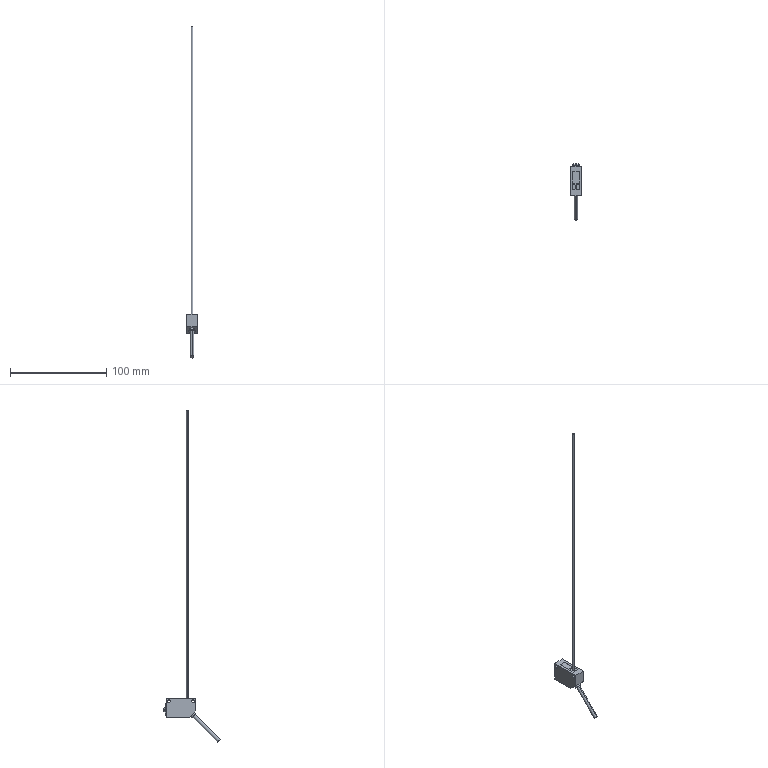Part | STEP file | 1 solid | 83 faces | box 11.2 x 58.715 x 345.215 mm | volume 7993 mm3 | plane 46 | cylinder 26 | cone 7 | sphere 4 | commonest cylinder face diameters 3.6 x10 2.92 x4 3 x4 2 x2 3.4 x2 3.7 x2